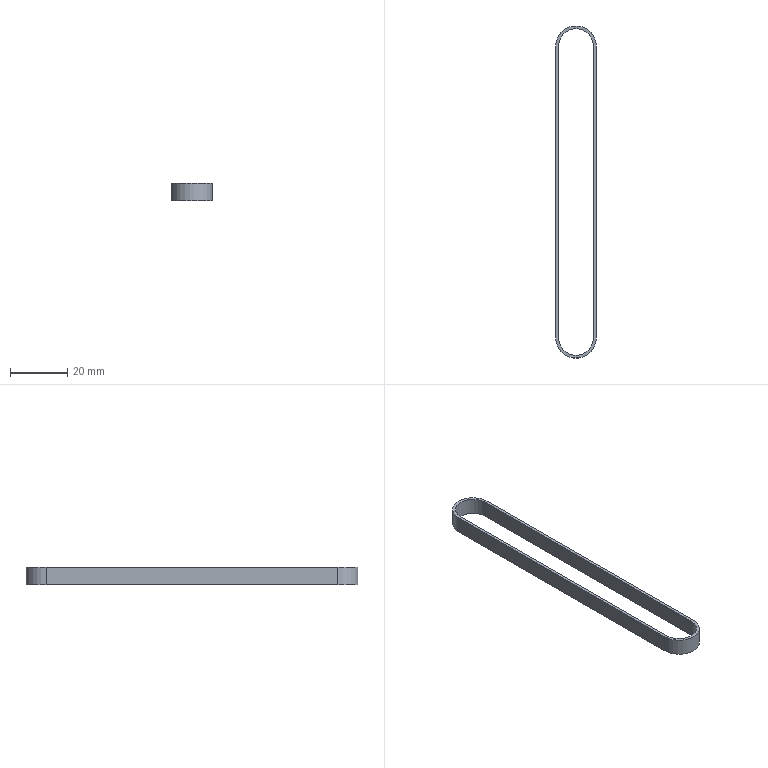Part | SolidWorks | features BaseBody 1 | 1 solid | 10 faces | box 14.22 x 116.22 x 6 mm | volume 1473 mm3 | plane 6 | cylinder 4 | commonest cylinder face diameters 12.22 x2 14.22 x2
STEP:
#1=CARTESIAN_POINT('',(35.61,48.,0.));
#2=VERTEX_POINT('',#1);
#3=CARTESIAN_POINT('',(35.61,48.,6.));
#4=VERTEX_POINT('',#3);
#5=CARTESIAN_POINT('',(35.61,48.,0.));
#6=DIRECTION('',(0.,0.,1.));
#7=VECTOR('',#6,1000.);
#8=LINE('',#5,#7);
#9=EDGE_CURVE('',#2,#4,#8,.T.);
#10=ORIENTED_EDGE('',*,*,#9,.F.);
#11=CARTESIAN_POINT('',(35.61,-54.,0.));
#12=VERTEX_POINT('',#11);
#13=CARTESIAN_POINT('',(35.61,48.,0.));
#14=DIRECTION('',(0.,1.,0.));
#15=VECTOR('',#14,1000.);
#16=LINE('',#13,#15);
#17=EDGE_CURVE('',#12,#2,#16,.T.);
#18=ORIENTED_EDGE('',*,*,#17,.F.);
#19=CARTESIAN_POINT('',(35.61,-54.,6.));
#20=VERTEX_POINT('',#19);
#21=CARTESIAN_POINT('',(35.61,-54.,0.));
#22=DIRECTION('',(0.,0.,-1.));
#23=VECTOR('',#22,1000.);
#24=LINE('',#21,#23);
#25=EDGE_CURVE('',#20,#12,#24,.T.);
#26=ORIENTED_EDGE('',*,*,#25,.F.);
#27=CARTESIAN_POINT('',(35.61,48.,6.));
#28=DIRECTION('',(0.,-1.,0.));
#29=VECTOR('',#28,1000.);
#30=LINE('',#27,#29);
#31=EDGE_CURVE('',#4,#20,#30,.T.);
#32=ORIENTED_EDGE('',*,*,#31,.F.);
#33=EDGE_LOOP('',(#10,#18,#26,#32));
#34=FACE_OUTER_BOUND('',#33,.T.);
#35=CARTESIAN_POINT('',(35.61,48.,0.));
#36=DIRECTION('',(1.,0.,0.));
#37=DIRECTION('',(0.,0.,-1.));
#38=AXIS2_PLACEMENT_3D('',#35,#36,#37);
#39=PLANE('',#38);
#40=ADVANCED_FACE('',(#34),#39,.F.);
#41=CARTESIAN_POINT('',(23.39,-54.,6.));
#42=VERTEX_POINT('',#41);
#43=CARTESIAN_POINT('',(29.5,-54.,6.));
#44=DIRECTION('',(0.,0.,-1.));
#45=DIRECTION('',(1.,0.,0.));
#46=AXIS2_PLACEMENT_3D('',#43,#44,#45);
#47=CIRCLE('',#46,6.11);
#48=EDGE_CURVE('',#20,#42,#47,.T.);
#49=ORIENTED_EDGE('',*,*,#48,.T.);
#50=CARTESIAN_POINT('',(23.39,48.,6.));
#51=VERTEX_POINT('',#50);
#52=CARTESIAN_POINT('',(23.39,-3.,6.));
#53=DIRECTION('',(0.,1.,0.));
#54=VECTOR('',#53,1000.);
#55=LINE('',#52,#54);
#56=EDGE_CURVE('',#42,#51,#55,.T.);
#57=ORIENTED_EDGE('',*,*,#56,.T.);
#58=CARTESIAN_POINT('',(29.5,48.,6.));
#59=DIRECTION('',(0.,0.,-1.));
#60=DIRECTION('',(1.,0.,0.));
#61=AXIS2_PLACEMENT_3D('',#58,#59,#60);
#62=CIRCLE('',#61,6.11);
#63=EDGE_CURVE('',#51,#4,#62,.T.);
#64=ORIENTED_EDGE('',*,*,#63,.T.);
#65=ORIENTED_EDGE('',*,*,#31,.T.);
#66=EDGE_LOOP('',(#49,#57,#64,#65));
#67=FACE_BOUND('',#66,.T.);
#68=CARTESIAN_POINT('',(36.61,48.,6.));
#69=VERTEX_POINT('',#68);
#70=CARTESIAN_POINT('',(22.39,48.,6.));
#71=VERTEX_POINT('',#70);
#72=CARTESIAN_POINT('',(29.5,48.,6.));
#73=DIRECTION('',(0.,0.,1.));
#74=DIRECTION('',(1.,0.,0.));
#75=AXIS2_PLACEMENT_3D('',#72,#73,#74);
#76=CIRCLE('',#75,7.11);
#77=EDGE_CURVE('',#69,#71,#76,.T.);
#78=ORIENTED_EDGE('',*,*,#77,.T.);
#79=CARTESIAN_POINT('',(22.39,-54.,6.));
#80=VERTEX_POINT('',#79);
#81=CARTESIAN_POINT('',(22.39,-3.,6.));
#82=DIRECTION('',(0.,-1.,0.));
#83=VECTOR('',#82,1000.);
#84=LINE('',#81,#83);
#85=EDGE_CURVE('',#71,#80,#84,.T.);
#86=ORIENTED_EDGE('',*,*,#85,.T.);
#87=CARTESIAN_POINT('',(36.61,-54.,6.));
#88=VERTEX_POINT('',#87);
#89=CARTESIAN_POINT('',(29.5,-54.,6.));
#90=DIRECTION('',(0.,0.,1.));
#91=DIRECTION('',(1.,0.,0.));
#92=AXIS2_PLACEMENT_3D('',#89,#90,#91);
#93=CIRCLE('',#92,7.11);
#94=EDGE_CURVE('',#80,#88,#93,.T.);
#95=ORIENTED_EDGE('',*,*,#94,.T.);
#96=CARTESIAN_POINT('',(36.61,-3.,6.));
#97=DIRECTION('',(0.,1.,0.));
#98=VECTOR('',#97,1000.);
#99=LINE('',#96,#98);
#100=EDGE_CURVE('',#88,#69,#99,.T.);
#101=ORIENTED_EDGE('',*,*,#100,.T.);
#102=EDGE_LOOP('',(#78,#86,#95,#101));
#103=FACE_OUTER_BOUND('',#102,.T.);
#104=CARTESIAN_POINT('',(29.5,-3.,6.));
#105=DIRECTION('',(0.,0.,1.));
#106=DIRECTION('',(1.,0.,0.));
#107=AXIS2_PLACEMENT_3D('',#104,#105,#106);
#108=PLANE('',#107);
#109=ADVANCED_FACE('',(#67,#103),#108,.T.);
#110=CARTESIAN_POINT('',(23.39,48.,0.));
#111=VERTEX_POINT('',#110);
#112=CARTESIAN_POINT('',(23.39,48.,0.));
#113=DIRECTION('',(0.,0.,1.));
#114=VECTOR('',#113,1000.);
#115=LINE('',#112,#114);
#116=EDGE_CURVE('',#111,#51,#115,.T.);
#117=ORIENTED_EDGE('',*,*,#116,.F.);
#118=CARTESIAN_POINT('',(29.5,48.,0.));
#119=DIRECTION('',(0.,0.,1.));
#120=DIRECTION('',(1.,0.,0.));
#121=AXIS2_PLACEMENT_3D('',#118,#119,#120);
#122=CIRCLE('',#121,6.11);
#123=EDGE_CURVE('',#2,#111,#122,.T.);
#124=ORIENTED_EDGE('',*,*,#123,.F.);
#125=ORIENTED_EDGE('',*,*,#9,.T.);
#126=ORIENTED_EDGE('',*,*,#63,.F.);
#127=EDGE_LOOP('',(#117,#124,#125,#126));
#128=FACE_OUTER_BOUND('',#127,.T.);
#129=CARTESIAN_POINT('',(29.5,48.,0.));
#130=DIRECTION('',(0.,0.,1.));
#131=DIRECTION('',(1.,0.,0.));
#132=AXIS2_PLACEMENT_3D('',#129,#130,#131);
#133=CYLINDRICAL_SURFACE('',#132,6.11);
#134=ADVANCED_FACE('',(#128),#133,.F.);
#135=CARTESIAN_POINT('',(23.39,-54.,0.));
#136=VERTEX_POINT('',#135);
#137=CARTESIAN_POINT('',(23.39,-3.,0.));
#138=DIRECTION('',(0.,1.,0.));
#139=VECTOR('',#138,1000.);
#140=LINE('',#137,#139);
#141=EDGE_CURVE('',#136,#111,#140,.T.);
#142=ORIENTED_EDGE('',*,*,#141,.F.);
#143=CARTESIAN_POINT('',(29.5,-54.,0.));
#144=DIRECTION('',(0.,0.,-1.));
#145=DIRECTION('',(1.,0.,0.));
#146=AXIS2_PLACEMENT_3D('',#143,#144,#145);
#147=CIRCLE('',#146,6.11);
#148=EDGE_CURVE('',#12,#136,#147,.T.);
#149=ORIENTED_EDGE('',*,*,#148,.F.);
#150=ORIENTED_EDGE('',*,*,#17,.T.);
#151=ORIENTED_EDGE('',*,*,#123,.T.);
#152=EDGE_LOOP('',(#142,#149,#150,#151));
#153=FACE_BOUND('',#152,.T.);
#154=CARTESIAN_POINT('',(22.39,-54.,0.));
#155=VERTEX_POINT('',#154);
#156=CARTESIAN_POINT('',(36.61,-54.,0.));
#157=VERTEX_POINT('',#156);
#158=CARTESIAN_POINT('',(29.5,-54.,0.));
#159=DIRECTION('',(0.,0.,1.));
#160=DIRECTION('',(1.,0.,0.));
#161=AXIS2_PLACEMENT_3D('',#158,#159,#160);
#162=CIRCLE('',#161,7.11);
#163=EDGE_CURVE('',#155,#157,#162,.T.);
#164=ORIENTED_EDGE('',*,*,#163,.F.);
#165=CARTESIAN_POINT('',(22.39,48.,0.));
#166=VERTEX_POINT('',#165);
#167=CARTESIAN_POINT('',(22.39,-3.,0.));
#168=DIRECTION('',(0.,-1.,0.));
#169=VECTOR('',#168,1000.);
#170=LINE('',#167,#169);
#171=EDGE_CURVE('',#166,#155,#170,.T.);
#172=ORIENTED_EDGE('',*,*,#171,.F.);
#173=CARTESIAN_POINT('',(36.61,48.,0.));
#174=VERTEX_POINT('',#173);
#175=CARTESIAN_POINT('',(29.5,48.,0.));
#176=DIRECTION('',(0.,0.,1.));
#177=DIRECTION('',(1.,0.,0.));
#178=AXIS2_PLACEMENT_3D('',#175,#176,#177);
#179=CIRCLE('',#178,7.11);
#180=EDGE_CURVE('',#174,#166,#179,.T.);
#181=ORIENTED_EDGE('',*,*,#180,.F.);
#182=CARTESIAN_POINT('',(36.61,-3.,0.));
#183=DIRECTION('',(0.,1.,0.));
#184=VECTOR('',#183,1000.);
#185=LINE('',#182,#184);
#186=EDGE_CURVE('',#157,#174,#185,.T.);
#187=ORIENTED_EDGE('',*,*,#186,.F.);
#188=EDGE_LOOP('',(#164,#172,#181,#187));
#189=FACE_OUTER_BOUND('',#188,.T.);
#190=CARTESIAN_POINT('',(29.5,-3.,0.));
#191=DIRECTION('',(0.,0.,1.));
#192=DIRECTION('',(1.,0.,0.));
#193=AXIS2_PLACEMENT_3D('',#190,#191,#192);
#194=PLANE('',#193);
#195=ADVANCED_FACE('',(#153,#189),#194,.F.);
#196=ORIENTED_EDGE('',*,*,#25,.T.);
#197=ORIENTED_EDGE('',*,*,#148,.T.);
#198=CARTESIAN_POINT('',(23.39,-54.,0.));
#199=DIRECTION('',(0.,0.,-1.));
#200=VECTOR('',#199,1000.);
#201=LINE('',#198,#200);
#202=EDGE_CURVE('',#42,#136,#201,.T.);
#203=ORIENTED_EDGE('',*,*,#202,.F.);
#204=ORIENTED_EDGE('',*,*,#48,.F.);
#205=EDGE_LOOP('',(#196,#197,#203,#204));
#206=FACE_OUTER_BOUND('',#205,.T.);
#207=CARTESIAN_POINT('',(29.5,-54.,0.));
#208=DIRECTION('',(0.,0.,1.));
#209=DIRECTION('',(1.,0.,0.));
#210=AXIS2_PLACEMENT_3D('',#207,#208,#209);
#211=CYLINDRICAL_SURFACE('',#210,6.11);
#212=ADVANCED_FACE('',(#206),#211,.F.);
#213=ORIENTED_EDGE('',*,*,#202,.T.);
#214=ORIENTED_EDGE('',*,*,#141,.T.);
#215=ORIENTED_EDGE('',*,*,#116,.T.);
#216=ORIENTED_EDGE('',*,*,#56,.F.);
#217=EDGE_LOOP('',(#213,#214,#215,#216));
#218=FACE_OUTER_BOUND('',#217,.T.);
#219=CARTESIAN_POINT('',(23.39,-54.,0.));
#220=DIRECTION('',(-1.,0.,0.));
#221=DIRECTION('',(0.,0.,1.));
#222=AXIS2_PLACEMENT_3D('',#219,#220,#221);
#223=PLANE('',#222);
#224=ADVANCED_FACE('',(#218),#223,.F.);
#225=ORIENTED_EDGE('',*,*,#171,.T.);
#226=CARTESIAN_POINT('',(22.39,-54.,0.));
#227=DIRECTION('',(0.,0.,1.));
#228=VECTOR('',#227,1000.);
#229=LINE('',#226,#228);
#230=EDGE_CURVE('',#155,#80,#229,.T.);
#231=ORIENTED_EDGE('',*,*,#230,.T.);
#232=ORIENTED_EDGE('',*,*,#85,.F.);
#233=CARTESIAN_POINT('',(22.39,48.,0.));
#234=DIRECTION('',(0.,0.,-1.));
#235=VECTOR('',#234,1000.);
#236=LINE('',#233,#235);
#237=EDGE_CURVE('',#71,#166,#236,.T.);
#238=ORIENTED_EDGE('',*,*,#237,.T.);
#239=EDGE_LOOP('',(#225,#231,#232,#238));
#240=FACE_OUTER_BOUND('',#239,.T.);
#241=CARTESIAN_POINT('',(22.39,-54.,0.));
#242=DIRECTION('',(-1.,0.,0.));
#243=DIRECTION('',(0.,0.,1.));
#244=AXIS2_PLACEMENT_3D('',#241,#242,#243);
#245=PLANE('',#244);
#246=ADVANCED_FACE('',(#240),#245,.T.);
#247=ORIENTED_EDGE('',*,*,#180,.T.);
#248=ORIENTED_EDGE('',*,*,#237,.F.);
#249=ORIENTED_EDGE('',*,*,#77,.F.);
#250=CARTESIAN_POINT('',(36.61,48.,0.));
#251=DIRECTION('',(0.,0.,-1.));
#252=VECTOR('',#251,1000.);
#253=LINE('',#250,#252);
#254=EDGE_CURVE('',#69,#174,#253,.T.);
#255=ORIENTED_EDGE('',*,*,#254,.T.);
#256=EDGE_LOOP('',(#247,#248,#249,#255));
#257=FACE_OUTER_BOUND('',#256,.T.);
#258=CARTESIAN_POINT('',(29.5,48.,0.));
#259=DIRECTION('',(0.,0.,1.));
#260=DIRECTION('',(1.,0.,0.));
#261=AXIS2_PLACEMENT_3D('',#258,#259,#260);
#262=CYLINDRICAL_SURFACE('',#261,7.11);
#263=ADVANCED_FACE('',(#257),#262,.T.);
#264=ORIENTED_EDGE('',*,*,#186,.T.);
#265=ORIENTED_EDGE('',*,*,#254,.F.);
#266=ORIENTED_EDGE('',*,*,#100,.F.);
#267=CARTESIAN_POINT('',(36.61,-54.,0.));
#268=DIRECTION('',(0.,0.,-1.));
#269=VECTOR('',#268,1000.);
#270=LINE('',#267,#269);
#271=EDGE_CURVE('',#88,#157,#270,.T.);
#272=ORIENTED_EDGE('',*,*,#271,.T.);
#273=EDGE_LOOP('',(#264,#265,#266,#272));
#274=FACE_OUTER_BOUND('',#273,.T.);
#275=CARTESIAN_POINT('',(36.61,48.,0.));
#276=DIRECTION('',(1.,0.,0.));
#277=DIRECTION('',(0.,0.,-1.));
#278=AXIS2_PLACEMENT_3D('',#275,#276,#277);
#279=PLANE('',#278);
#280=ADVANCED_FACE('',(#274),#279,.T.);
#281=ORIENTED_EDGE('',*,*,#163,.T.);
#282=ORIENTED_EDGE('',*,*,#271,.F.);
#283=ORIENTED_EDGE('',*,*,#94,.F.);
#284=ORIENTED_EDGE('',*,*,#230,.F.);
#285=EDGE_LOOP('',(#281,#282,#283,#284));
#286=FACE_OUTER_BOUND('',#285,.T.);
#287=CARTESIAN_POINT('',(29.5,-54.,0.));
#288=DIRECTION('',(0.,0.,1.));
#289=DIRECTION('',(1.,0.,0.));
#290=AXIS2_PLACEMENT_3D('',#287,#288,#289);
#291=CYLINDRICAL_SURFACE('',#290,7.11);
#292=ADVANCED_FACE('',(#286),#291,.T.);
#293=CLOSED_SHELL('',(#40,#109,#134,#195,#212,#224,#246,#263,#280,#292));
#294=MANIFOLD_SOLID_BREP('',#293);
#295=CARTESIAN_POINT('',(0.,0.,0.));
#296=DIRECTION('',(0.,0.,1.));
#297=DIRECTION('',(1.,0.,0.));
#298=AXIS2_PLACEMENT_3D('',#295,#296,#297);
#299=(LENGTH_UNIT()NAMED_UNIT(*)SI_UNIT(.MILLI.,.METRE.));
#300=UNCERTAINTY_MEASURE_WITH_UNIT(LENGTH_MEASURE(0.00001),#299,'','');
#301=(NAMED_UNIT(*)PLANE_ANGLE_UNIT()SI_UNIT($,.RADIAN.));
#302=(NAMED_UNIT(*)SI_UNIT($,.STERADIAN.)SOLID_ANGLE_UNIT());
#303=(GEOMETRIC_REPRESENTATION_CONTEXT(3)GLOBAL_UNCERTAINTY_ASSIGNED_CONTEXT((#300))GLOBAL_UNIT_ASSIGNED_CONTEXT((#299,#301,#302))REPRESENTATION_CONTEXT('',''));
#304=ADVANCED_BREP_SHAPE_REPRESENTATION('',(#294,#298),#303);